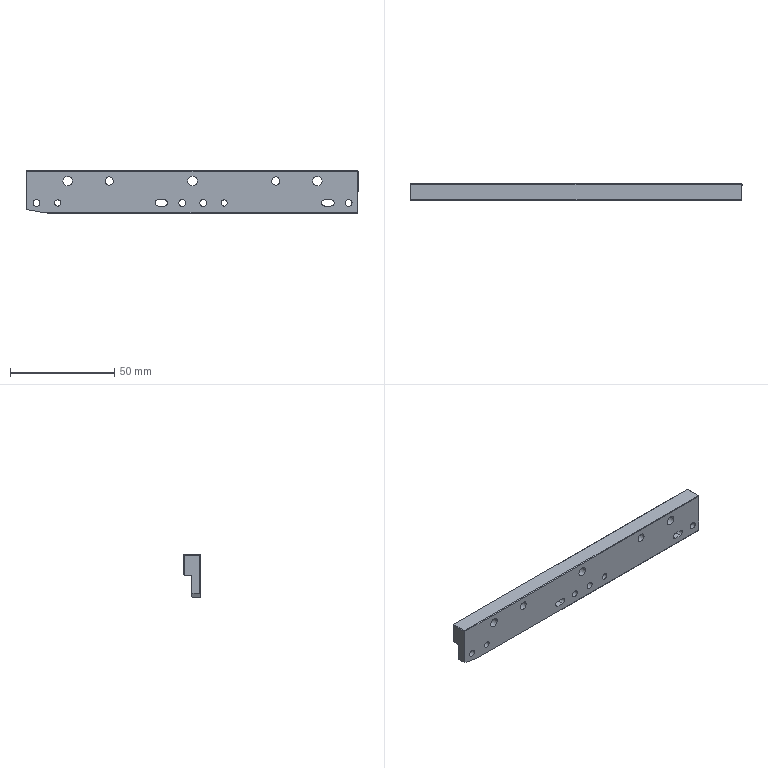Part | NX | 1 solid | 71 faces | box 159.5 x 8 x 20.5 mm | volume 18627 mm3 | cylinder 28 | plane 25 | cone 18 | commonest cylinder face diameters 3 x10 3.3 x8 4.5 x6 4 x4